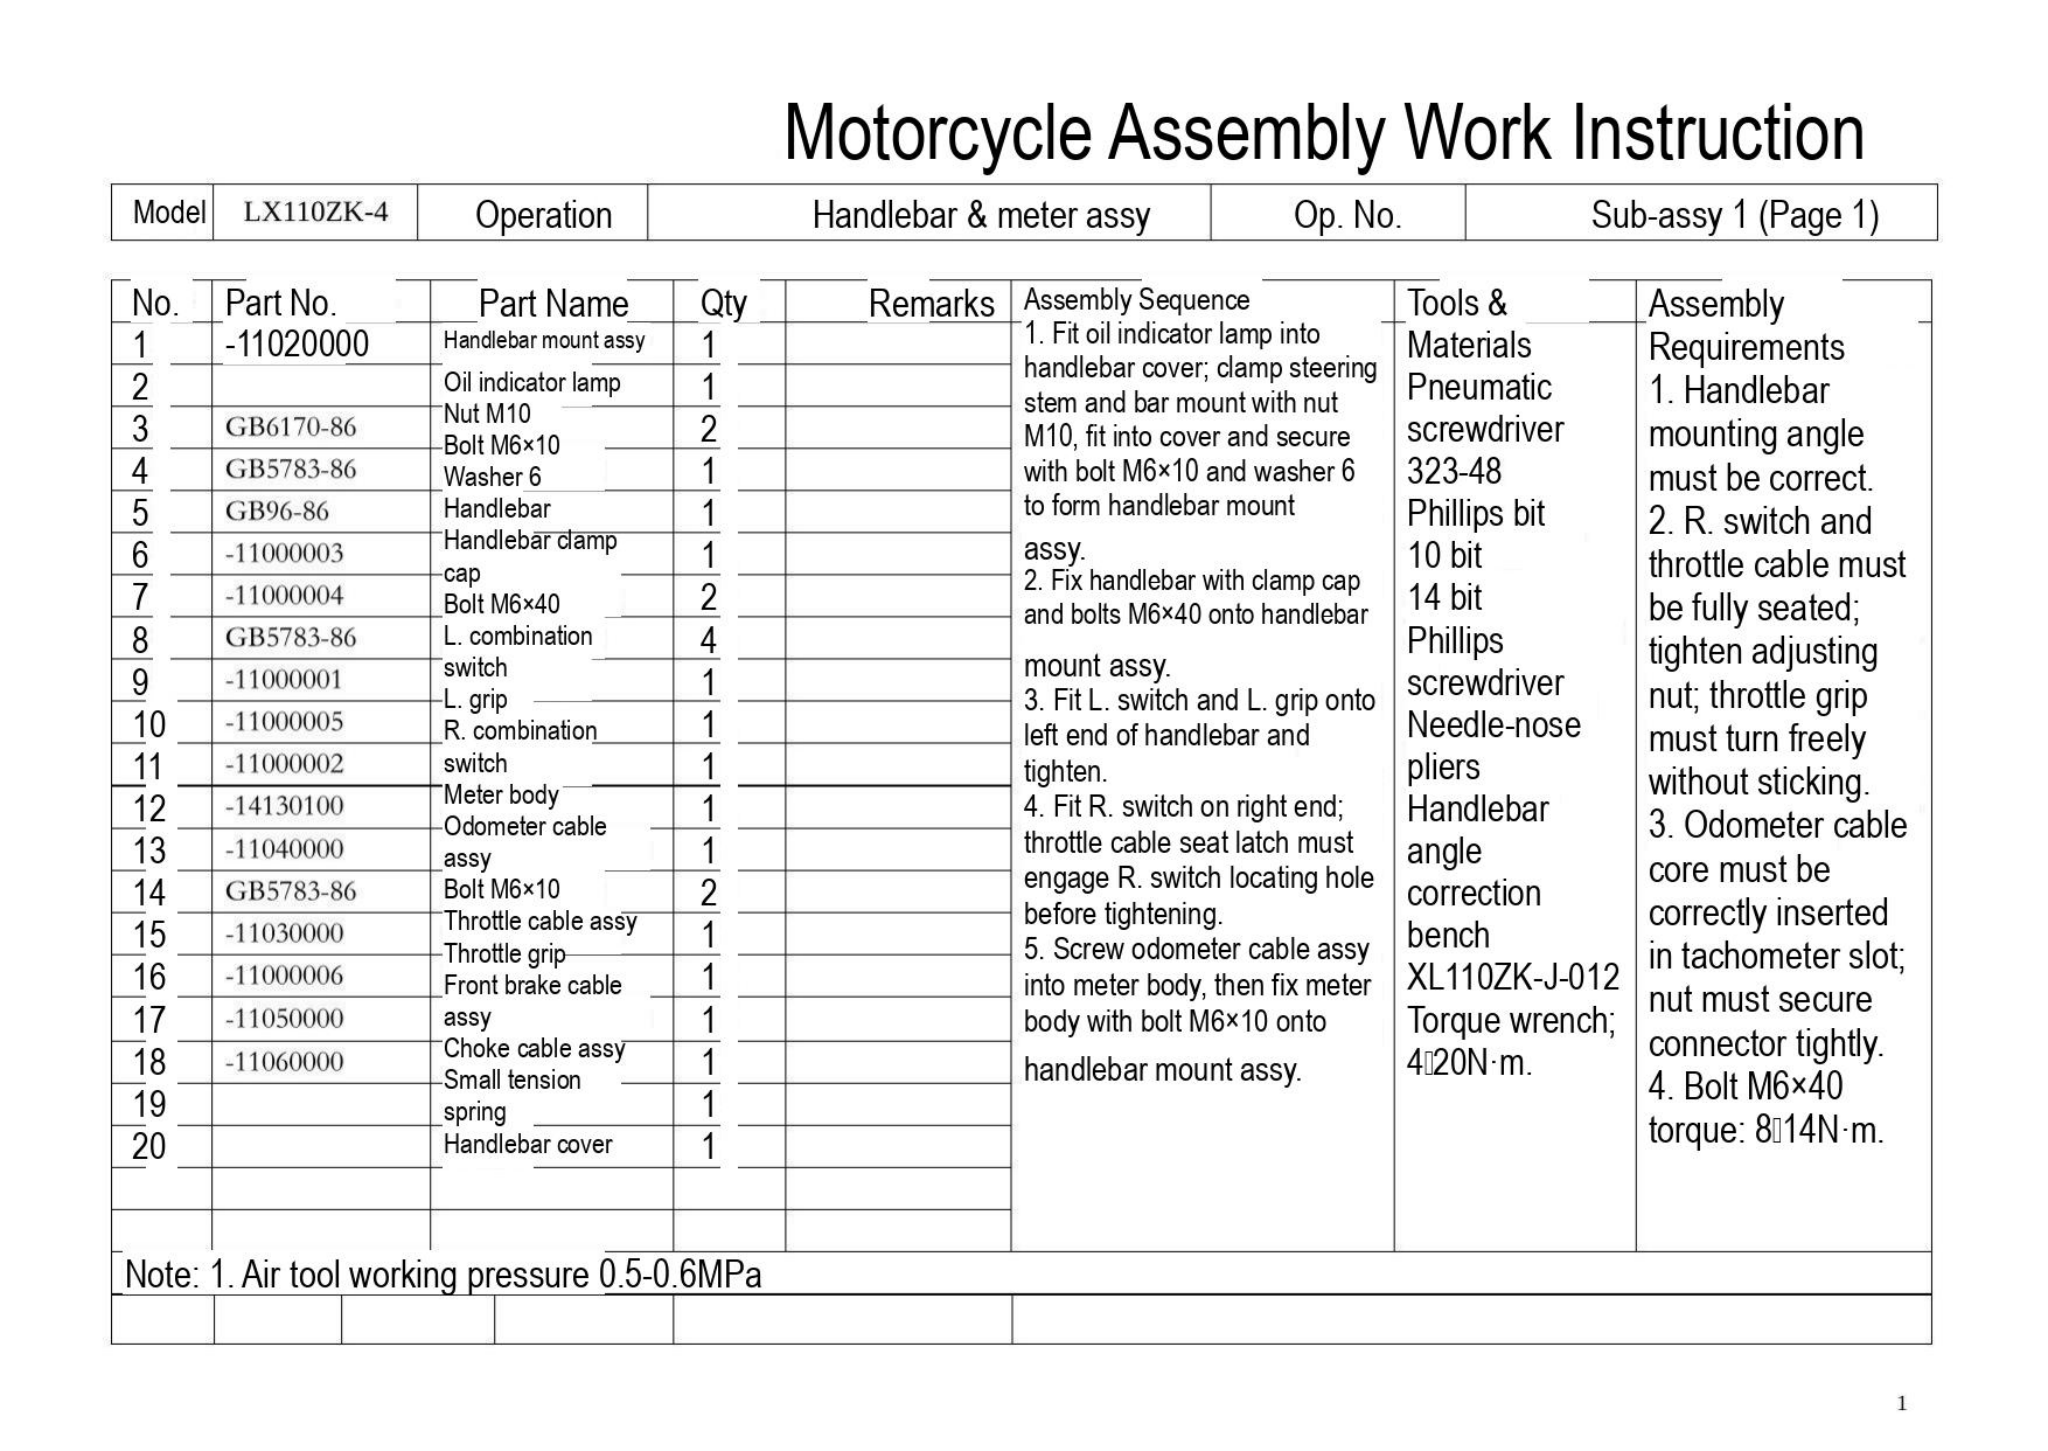# Motorcycle Assembly Work Instruction

| Model | LX110ZK-4 | Operation | Handlebar & meter assy | Op. No. | Sub-assy 1 (Page 1) |
|---|---|---|---|---|---|

| No. | Part No. | Part Name | Qty | Remarks |
|---|---|---|---|---|
| 1 | -11020000 | Handlebar mount assy | 1 | |
| 2 | | Oil indicator lamp | 1 | |
| 3 | GB6170-86 | Nut M10 | 2 | |
| 4 | GB5783-86 | Bolt M6×10 | 1 | |
| 5 | GB96-86 | Washer 6 | 1 | |
| 6 | -11000003 | Handlebar | 1 | |
| 7 | -11000004 | Handlebar clamp cap | 2 | |
| 8 | GB5783-86 | Bolt M6×40 | 4 | |
| 9 | -11000001 | L. combination switch | 1 | |
| 10 | -11000005 | L. grip | 1 | |
| 11 | -11000002 | R. combination switch | 1 | |
| 12 | -14130100 | Meter body | 1 | |
| 13 | -11040000 | Odometer cable assy | 1 | |
| 14 | GB5783-86 | Bolt M6×10 | 2 | |
| 15 | -11030000 | Throttle cable assy | 1 | |
| 16 | -11000006 | Throttle grip | 1 | |
| 17 | -11050000 | Front brake cable assy | 1 | |
| 18 | -11060000 | Choke cable assy | 1 | |
| 19 | | Small tension spring | 1 | |
| 20 | | Handlebar cover | 1 | |

**Assembly Sequence**
1. Fit oil indicator lamp into handlebar cover; clamp steering stem and bar mount with nut M10, fit into cover and secure with bolt M6×10 and washer 6 to form handlebar mount assy.
2. Fix handlebar with clamp cap and bolts M6×40 onto handlebar mount assy.
3. Fit L. switch and L. grip onto left end of handlebar and tighten.
4. Fit R. switch on right end; throttle cable seat latch must engage R. switch locating hole before tightening.
5. Screw odometer cable assy into meter body, then fix meter body with bolt M6×10 onto handlebar mount assy.

**Tools & Materials**
Pneumatic screwdriver 323-48
Phillips bit
10 bit
14 bit
Phillips screwdriver
Needle-nose pliers
Handlebar angle correction bench XL110ZK-J-012
Torque wrench; 4□20N·m.

**Assembly Requirements**
1. Handlebar mounting angle must be correct.
2. R. switch and throttle cable must be fully seated; tighten adjusting nut; throttle grip must turn freely without sticking.
3. Odometer cable core must be correctly inserted in tachometer slot; nut must secure connector tightly.
4. Bolt M6×40 torque: 8□14N·m.

Note: 1. Air tool working pressure 0.5-0.6MPa

1
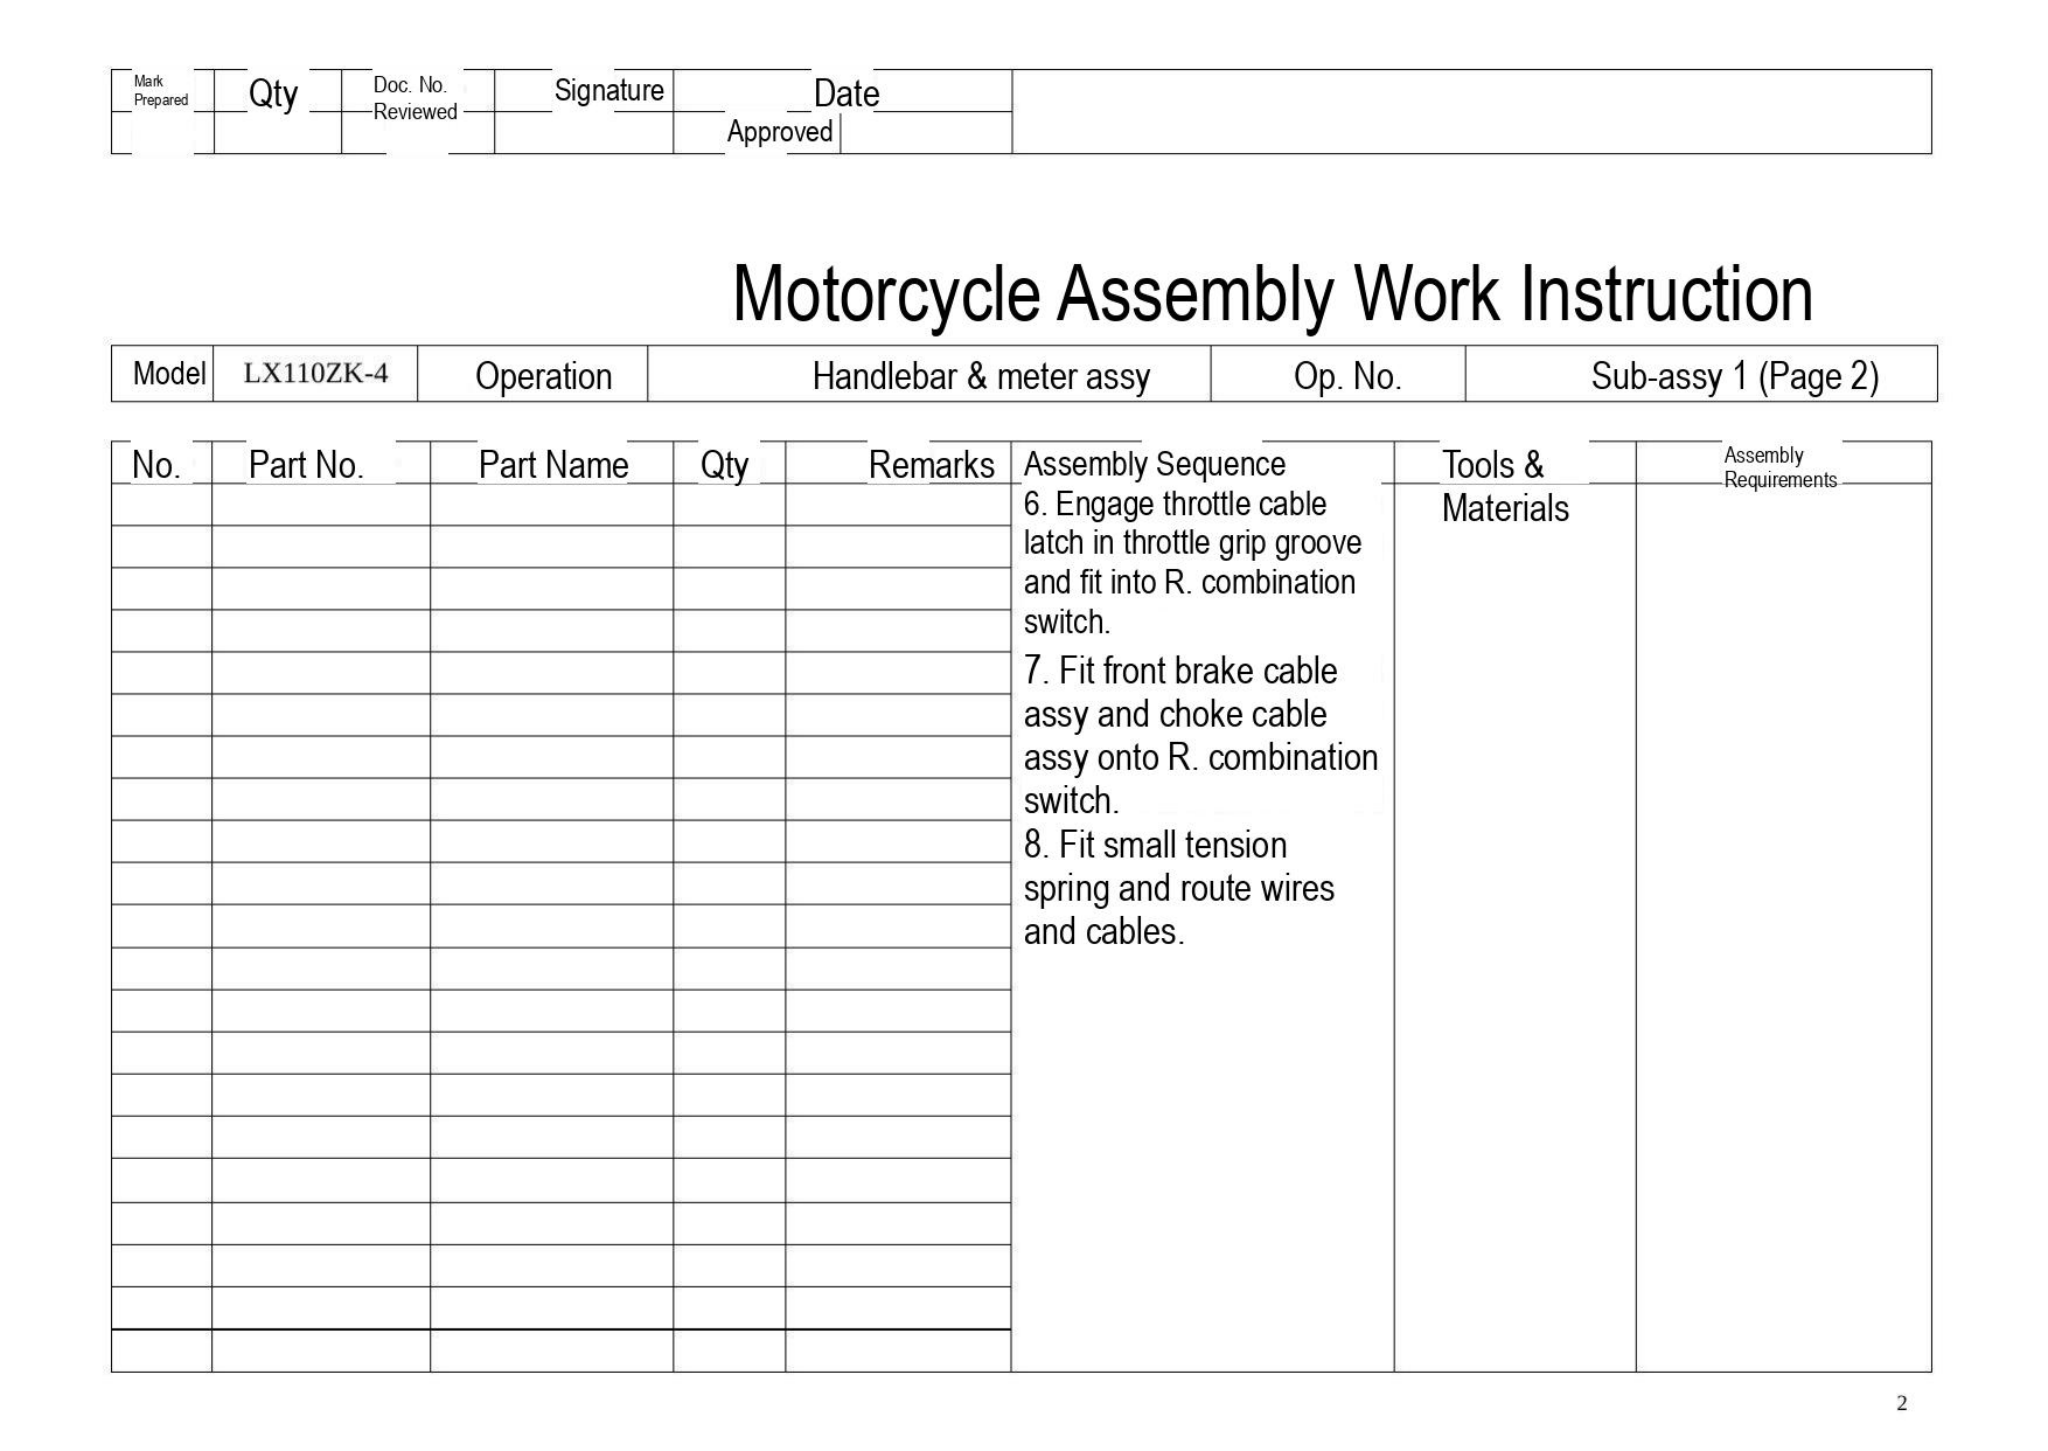| Mark Prepared | Qty | Doc. No. Reviewed | Signature | Date Approved | |
|---|---|---|---|---|---|
| | | | | | |

# Motorcycle Assembly Work Instruction

| Model | LX110ZK-4 | Operation | Handlebar & meter assy | Op. No. | Sub-assy 1 (Page 2) |
|---|---|---|---|---|---|

| No. | Part No. | Part Name | Qty | Remarks | Assembly Sequence | Tools & Materials | Assembly Requirements |
|---|---|---|---|---|---|---|---|
| | | | | | 6. Engage throttle cable latch in throttle grip groove and fit into R. combination switch.<br>7. Fit front brake cable assy and choke cable assy onto R. combination switch.<br>8. Fit small tension spring and route wires and cables. | | |

2
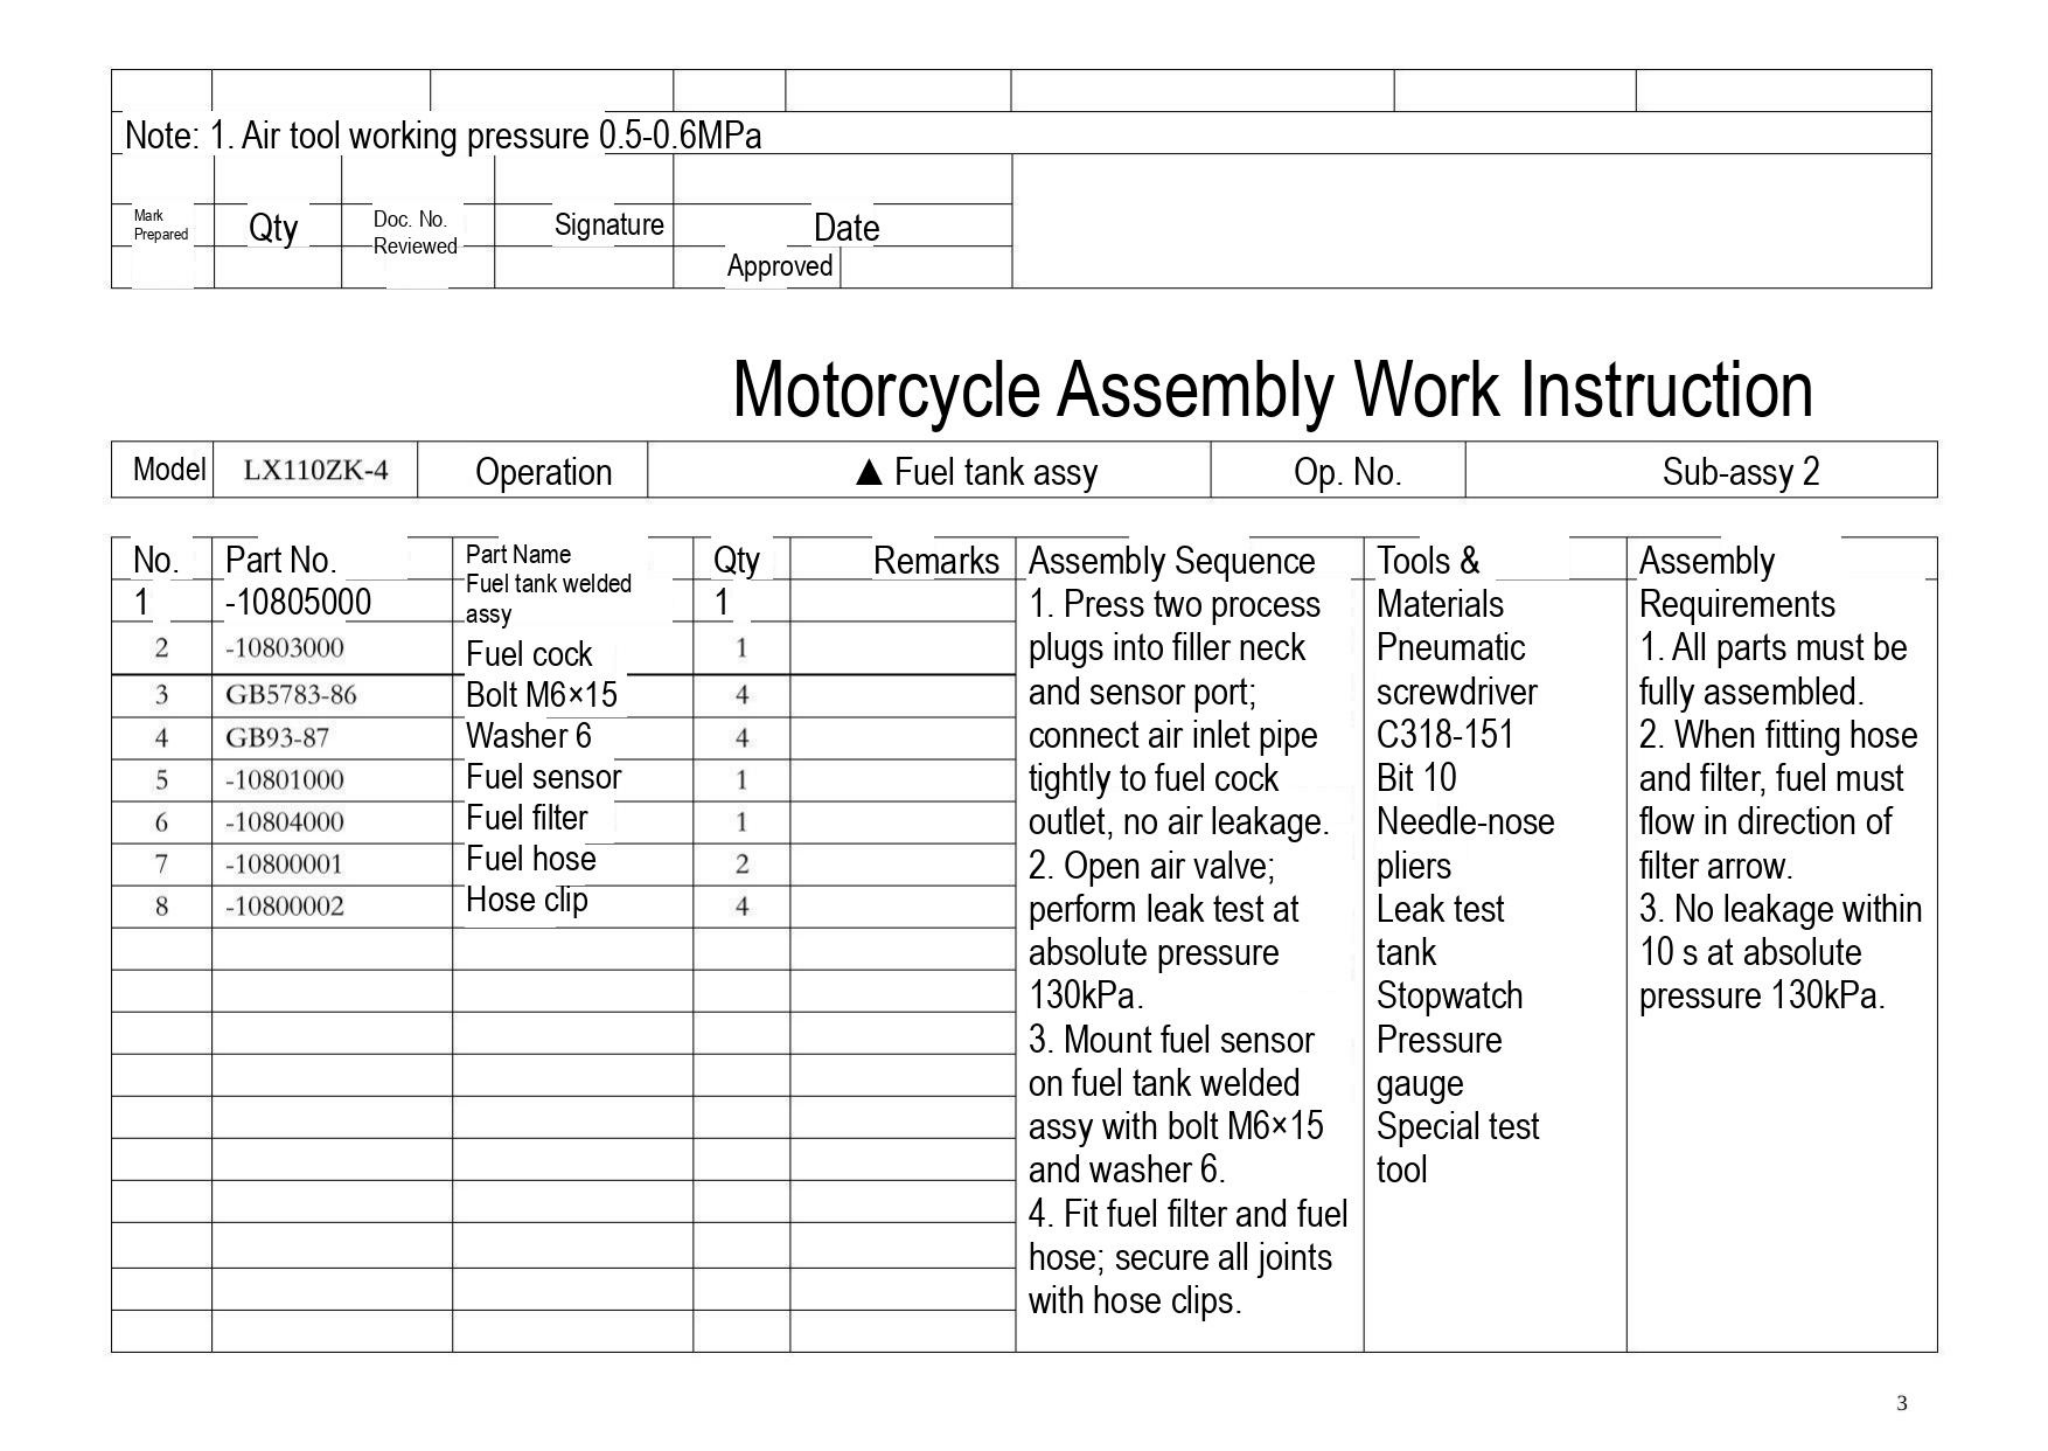| | | | | | | | |
|---|---|---|---|---|---|---|---|
| Note: 1. Air tool working pressure 0.5-0.6MPa | | | | | | | |
| Mark Prepared | Qty | Doc. No. Reviewed | Signature | Date Approved | | | |

# Motorcycle Assembly Work Instruction

| Model | LX110ZK-4 | Operation | ▲ Fuel tank assy | Op. No. | Sub-assy 2 |
|---|---|---|---|---|---|

| No. | Part No. | Part Name | Qty | Remarks | Assembly Sequence | Tools & Materials | Assembly Requirements |
|---|---|---|---|---|---|---|---|
| 1 | -10805000 | Fuel tank welded assy | 1 | | 1. Press two process plugs into filler neck and sensor port; connect air inlet pipe tightly to fuel cock outlet, no air leakage.<br>2. Open air valve; perform leak test at absolute pressure 130kPa.<br>3. Mount fuel sensor on fuel tank welded assy with bolt M6×15 and washer 6.<br>4. Fit fuel filter and fuel hose; secure all joints with hose clips. | Pneumatic screwdriver C318-151<br>Bit 10<br>Needle-nose pliers<br>Leak test tank<br>Stopwatch<br>Pressure gauge<br>Special test tool | 1. All parts must be fully assembled.<br>2. When fitting hose and filter, fuel must flow in direction of filter arrow.<br>3. No leakage within 10 s at absolute pressure 130kPa. |
| 2 | -10803000 | Fuel cock | 1 | | | | |
| 3 | GB5783-86 | Bolt M6×15 | 4 | | | | |
| 4 | GB93-87 | Washer 6 | 4 | | | | |
| 5 | -10801000 | Fuel sensor | 1 | | | | |
| 6 | -10804000 | Fuel filter | 1 | | | | |
| 7 | -10800001 | Fuel hose | 2 | | | | |
| 8 | -10800002 | Hose clip | 4 | | | | |

3
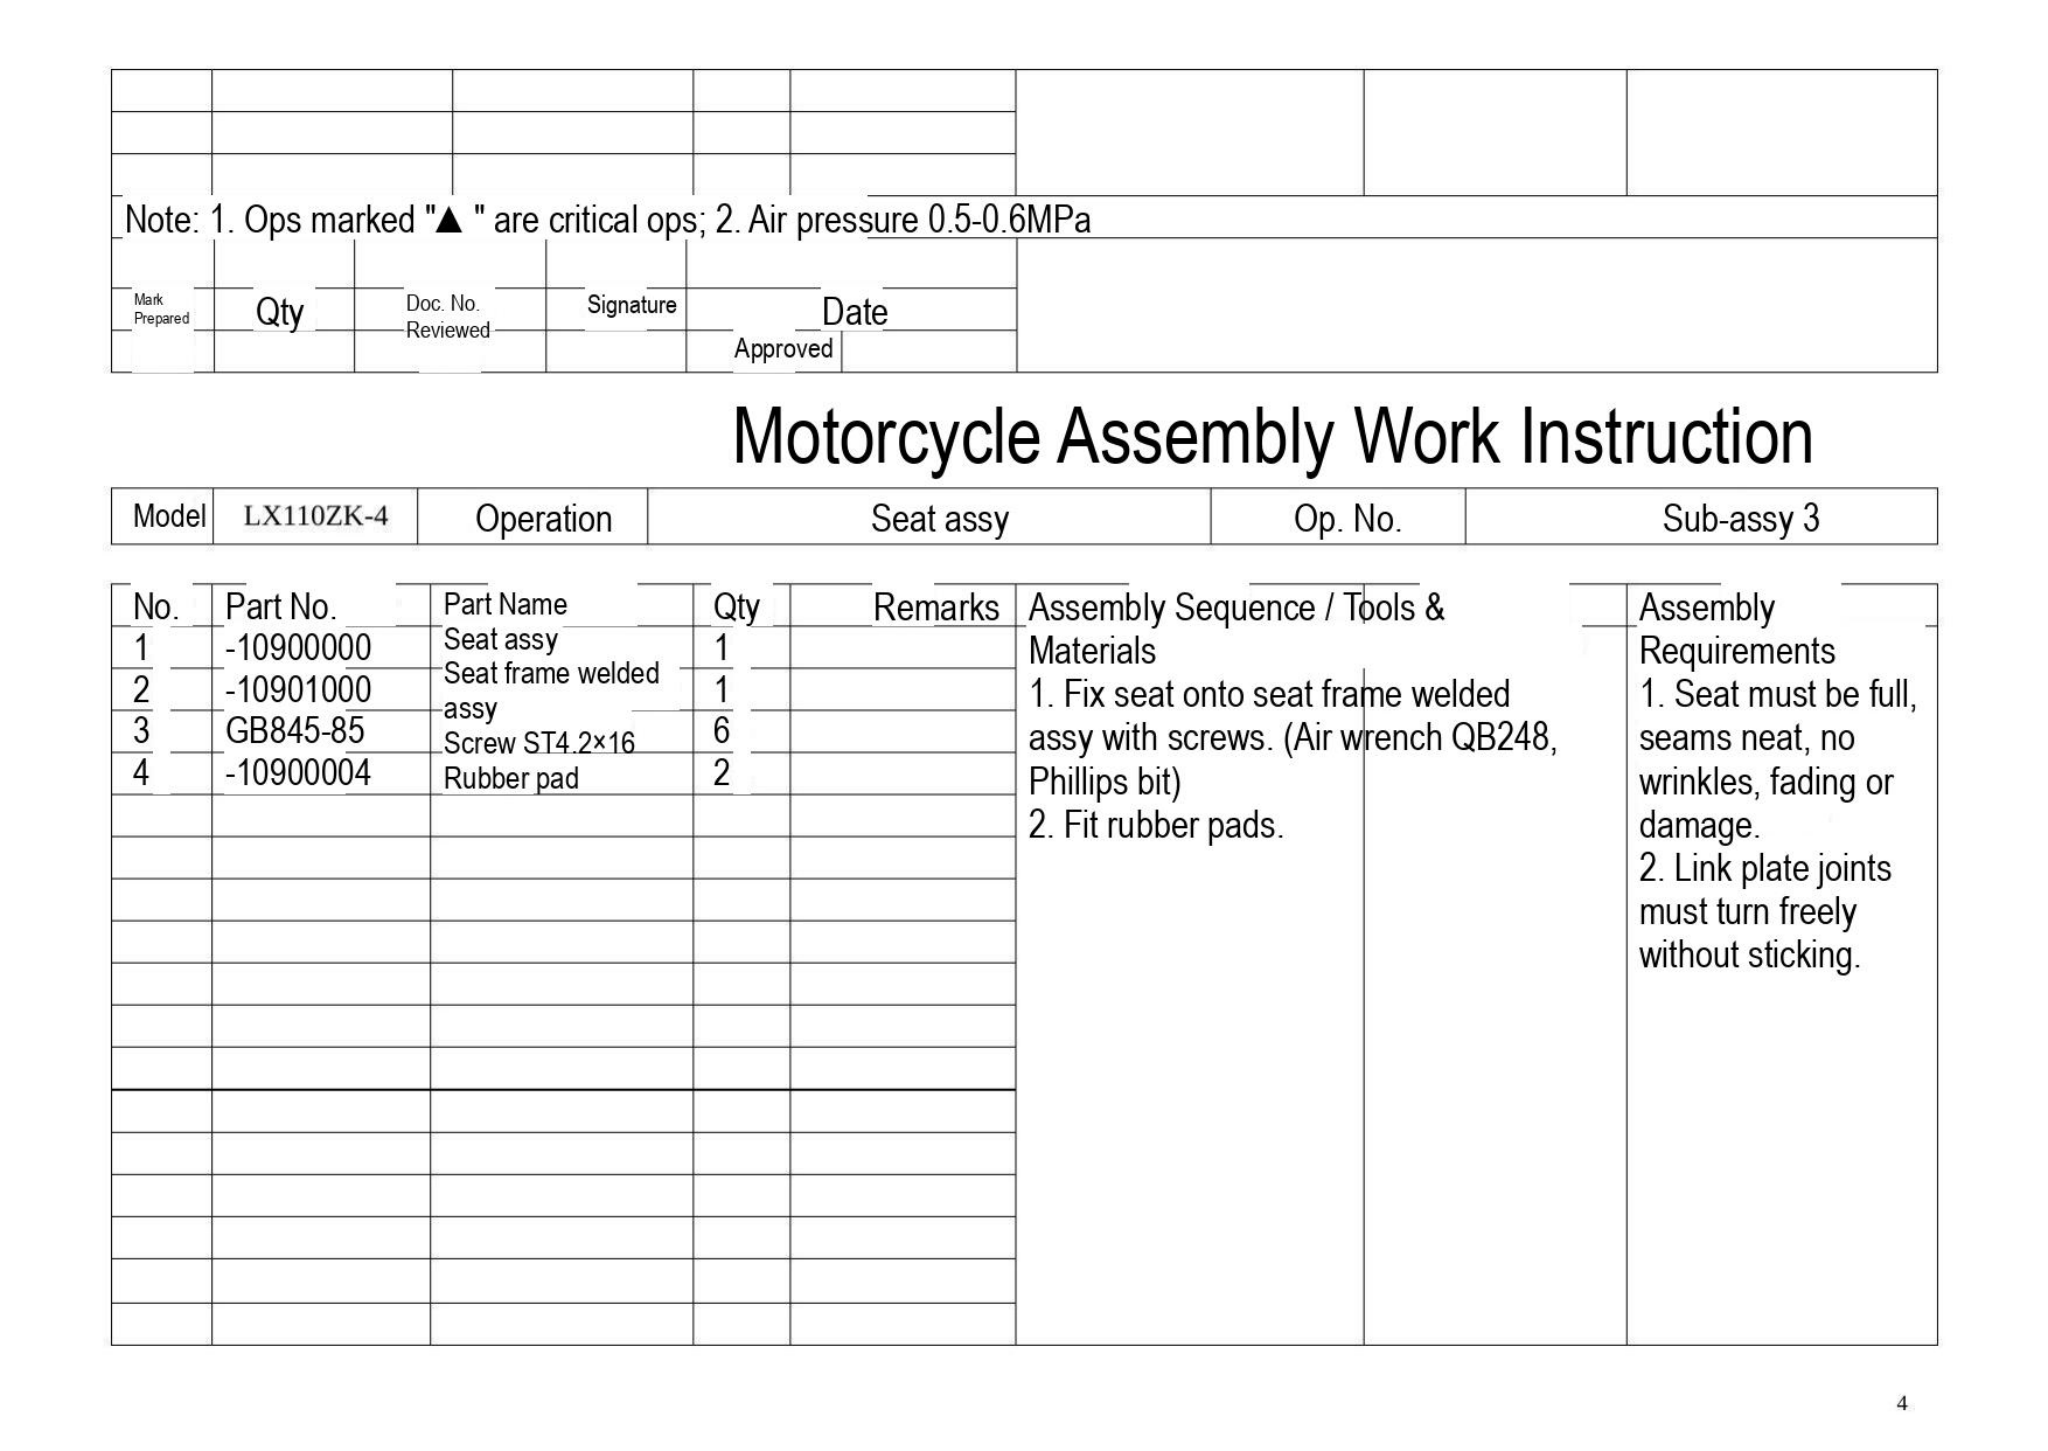Note: 1. Ops marked "▲ " are critical ops; 2. Air pressure 0.5-0.6MPa

| Mark Prepared | Qty | Doc. No. Reviewed | Signature | Date Approved |
|---|---|---|---|---|

# Motorcycle Assembly Work Instruction

| Model | LX110ZK-4 | Operation | Seat assy | Op. No. | Sub-assy 3 |
|---|---|---|---|---|---|

| No. | Part No. | Part Name | Qty | Remarks |
|---|---|---|---|---|
| 1 | -10900000 | Seat assy | 1 | |
| 2 | -10901000 | Seat frame welded assy | 1 | |
| 3 | GB845-85 | Screw ST4.2×16 | 6 | |
| 4 | -10900004 | Rubber pad | 2 | |

Assembly Sequence / Tools & Materials
1. Fix seat onto seat frame welded assy with screws. (Air wrench QB248, Phillips bit)
2. Fit rubber pads.

Assembly Requirements
1. Seat must be full, seams neat, no wrinkles, fading or damage.
2. Link plate joints must turn freely without sticking.

4
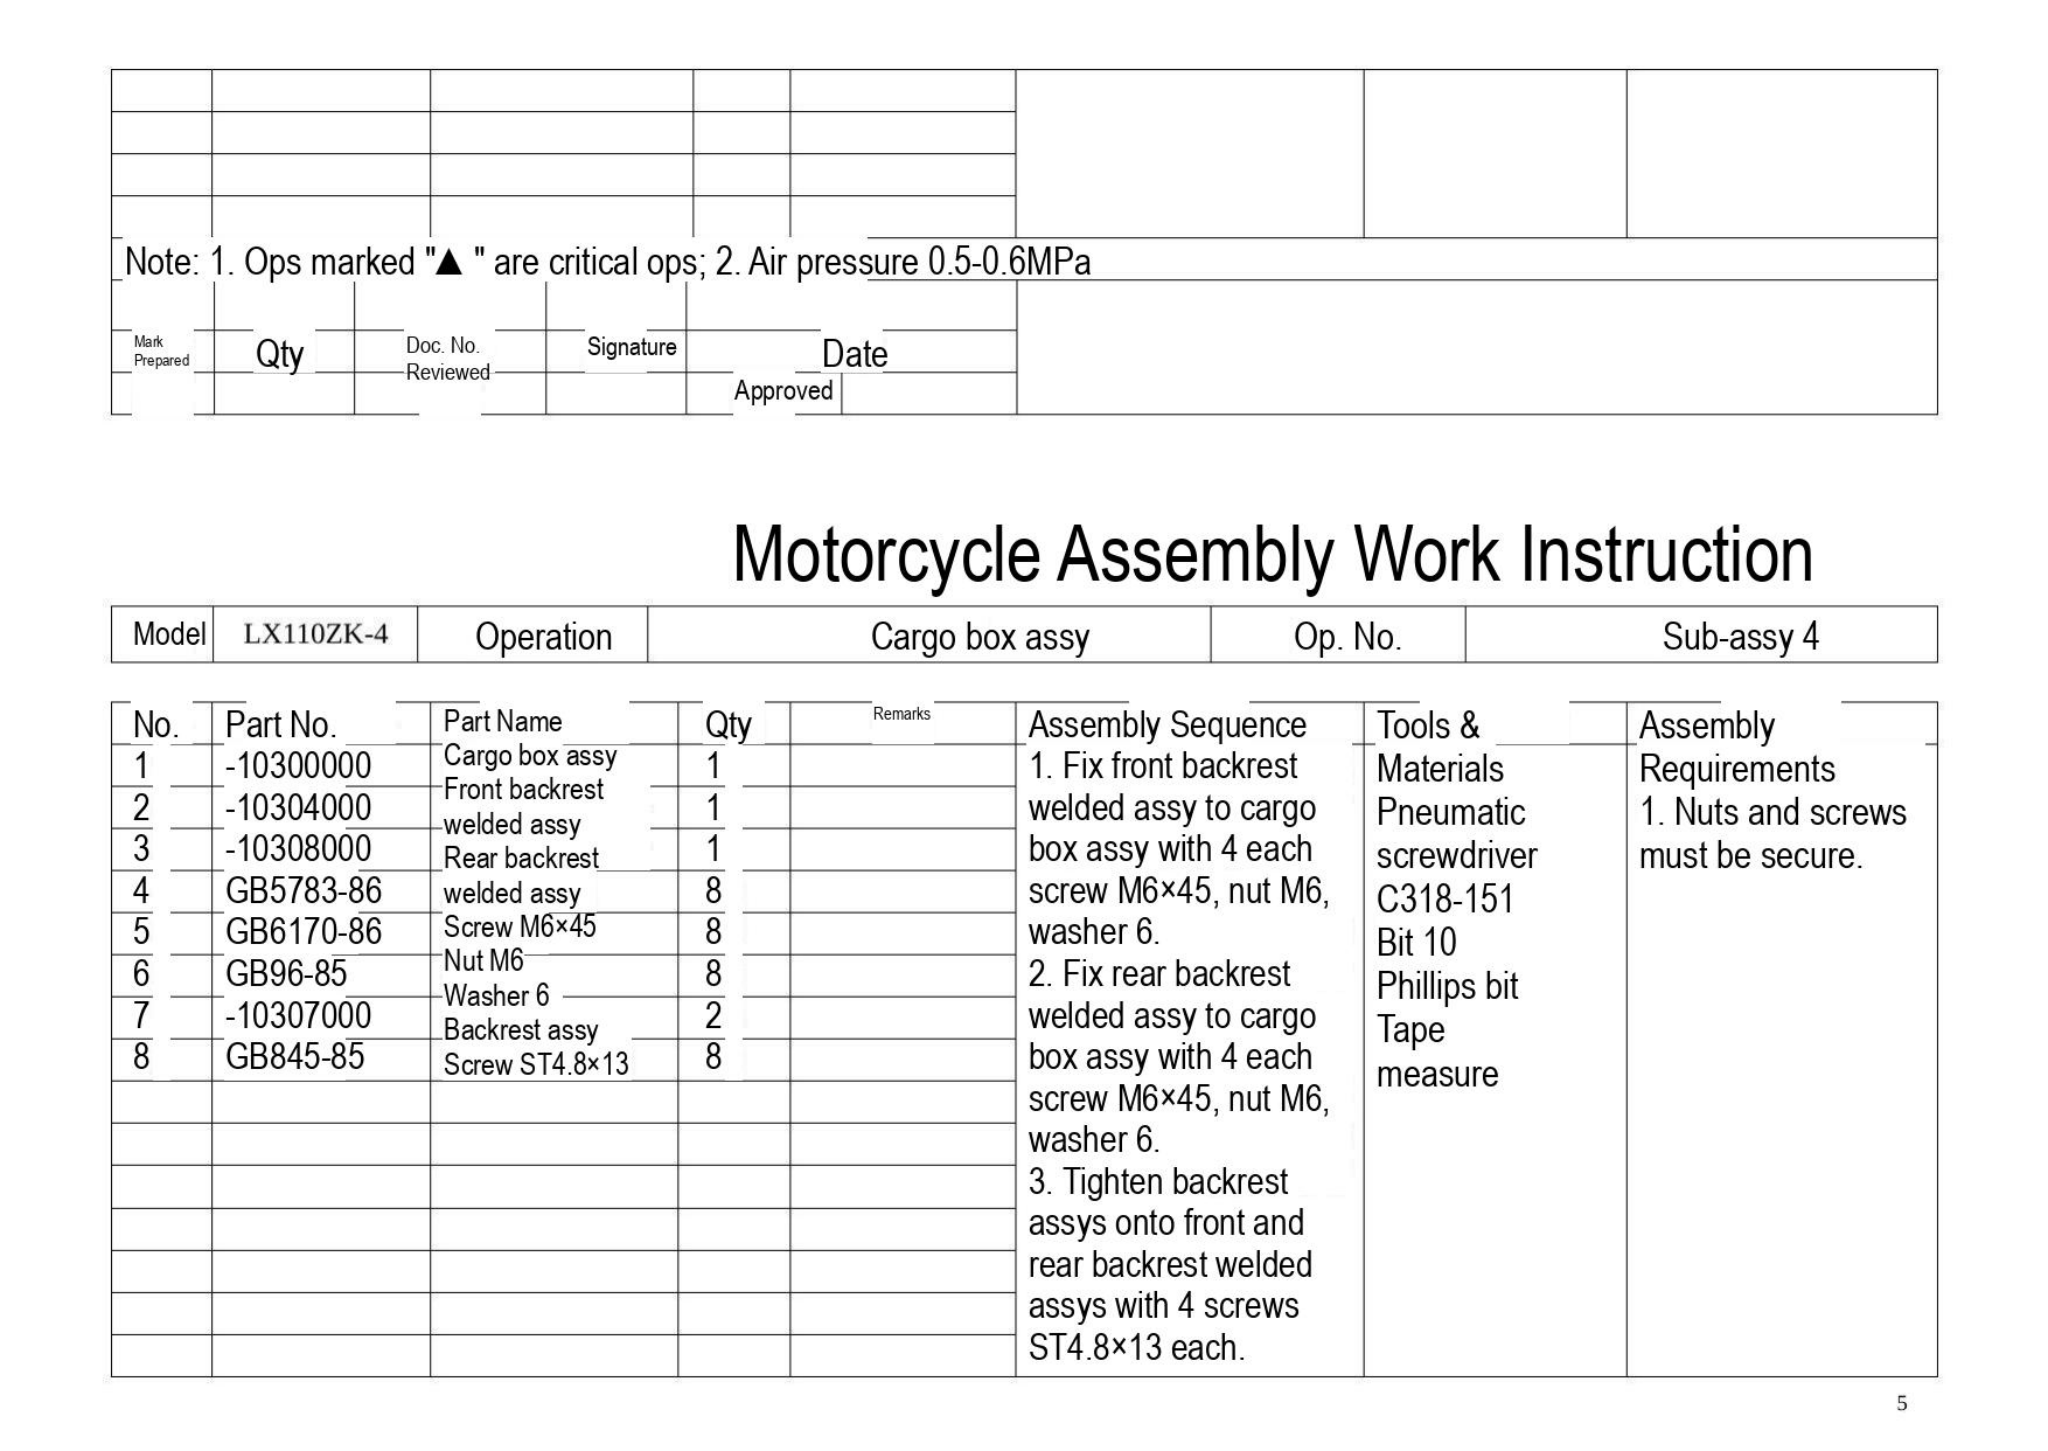Note: 1. Ops marked "▲ " are critical ops; 2. Air pressure 0.5-0.6MPa

| Mark Prepared | Qty | Doc. No. Reviewed | Signature | Date Approved |
|---|---|---|---|---|

# Motorcycle Assembly Work Instruction

| Model | LX110ZK-4 | Operation | Cargo box assy | Op. No. | Sub-assy 4 |
|---|---|---|---|---|---|

| No. | Part No. | Part Name | Qty | Remarks |
|---|---|---|---|---|
| 1 | -10300000 | Cargo box assy | 1 | |
| 2 | -10304000 | Front backrest welded assy | 1 | |
| 3 | -10308000 | Rear backrest welded assy | 1 | |
| 4 | GB5783-86 | Screw M6×45 | 8 | |
| 5 | GB6170-86 | Nut M6 | 8 | |
| 6 | GB96-85 | Washer 6 | 8 | |
| 7 | -10307000 | Backrest assy | 2 | |
| 8 | GB845-85 | Screw ST4.8×13 | 8 | |

Assembly Sequence
1. Fix front backrest welded assy to cargo box assy with 4 each screw M6×45, nut M6, washer 6.
2. Fix rear backrest welded assy to cargo box assy with 4 each screw M6×45, nut M6, washer 6.
3. Tighten backrest assys onto front and rear backrest welded assys with 4 screws ST4.8×13 each.

Tools & Materials
Pneumatic screwdriver C318-151
Bit 10
Phillips bit
Tape measure

Assembly Requirements
1. Nuts and screws must be secure.

5
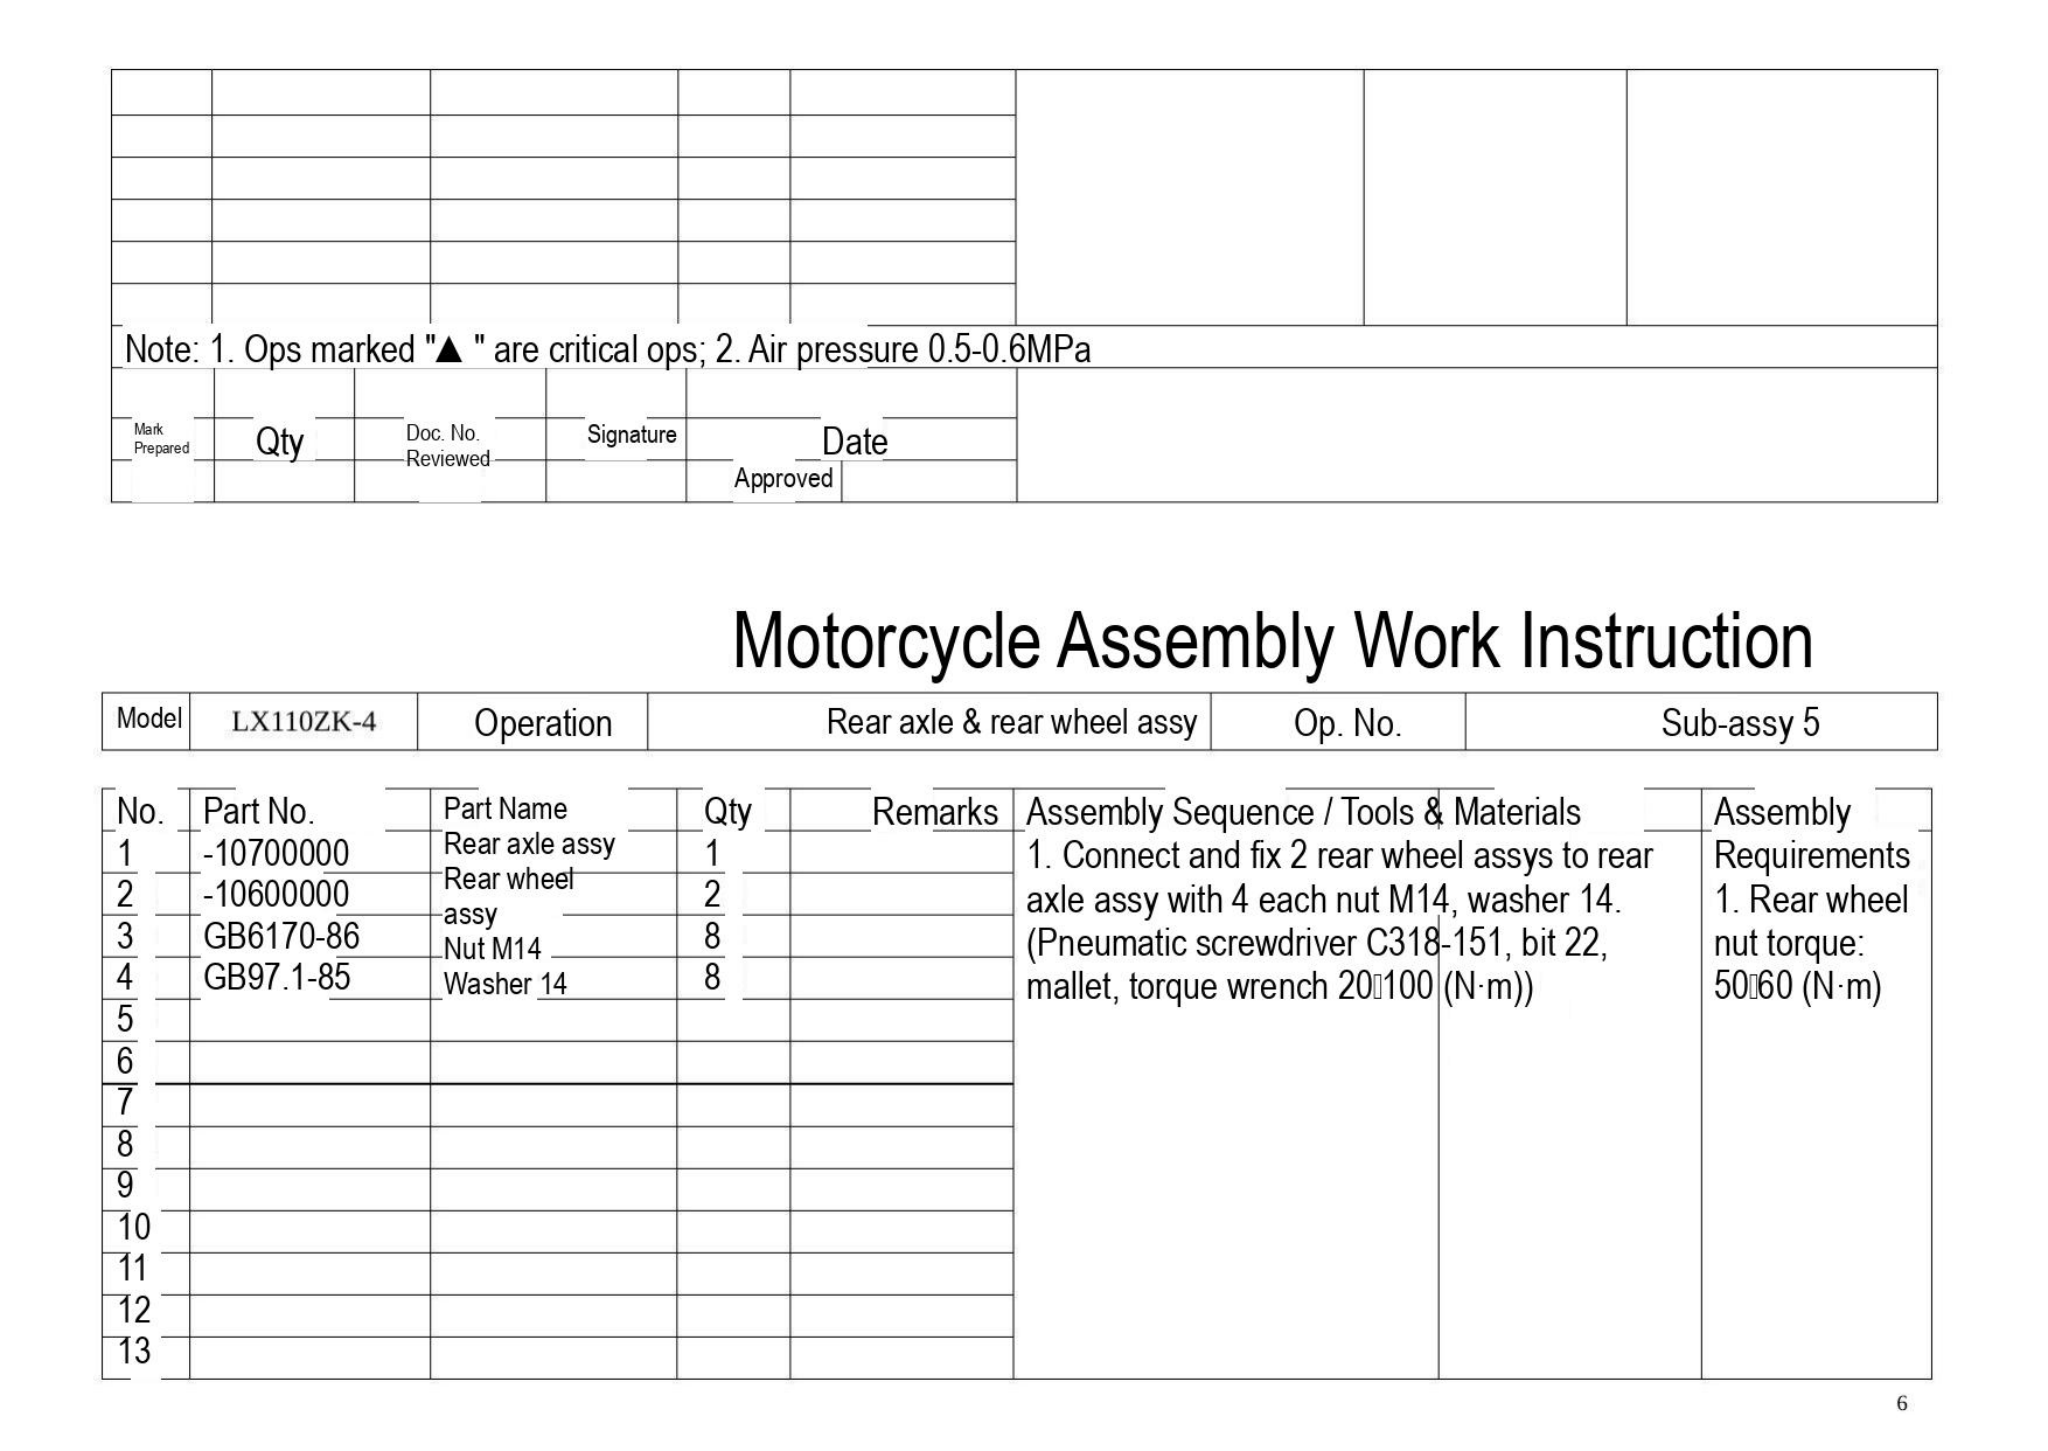Note: 1. Ops marked "▲ " are critical ops; 2. Air pressure 0.5-0.6MPa

| Mark Prepared | Qty | Doc. No. Reviewed | Signature | Date Approved |
|---|---|---|---|---|

# Motorcycle Assembly Work Instruction

| Model | LX110ZK-4 | Operation | Rear axle & rear wheel assy | Op. No. | Sub-assy 5 |
|---|---|---|---|---|---|

| No. | Part No. | Part Name | Qty | Remarks |
|---|---|---|---|---|
| 1 | -10700000 | Rear axle assy | 1 | |
| 2 | -10600000 | Rear wheel assy | 2 | |
| 3 | GB6170-86 | Nut M14 | 8 | |
| 4 | GB97.1-85 | Washer 14 | 8 | |
| 5 | | | | |
| 6 | | | | |
| 7 | | | | |
| 8 | | | | |
| 9 | | | | |
| 10 | | | | |
| 11 | | | | |
| 12 | | | | |
| 13 | | | | |

Assembly Sequence / Tools & Materials

1. Connect and fix 2 rear wheel assys to rear axle assy with 4 each nut M14, washer 14. (Pneumatic screwdriver C318-151, bit 22, mallet, torque wrench 20100 (N·m))

Assembly Requirements

1. Rear wheel nut torque: 5060 (N·m)

6
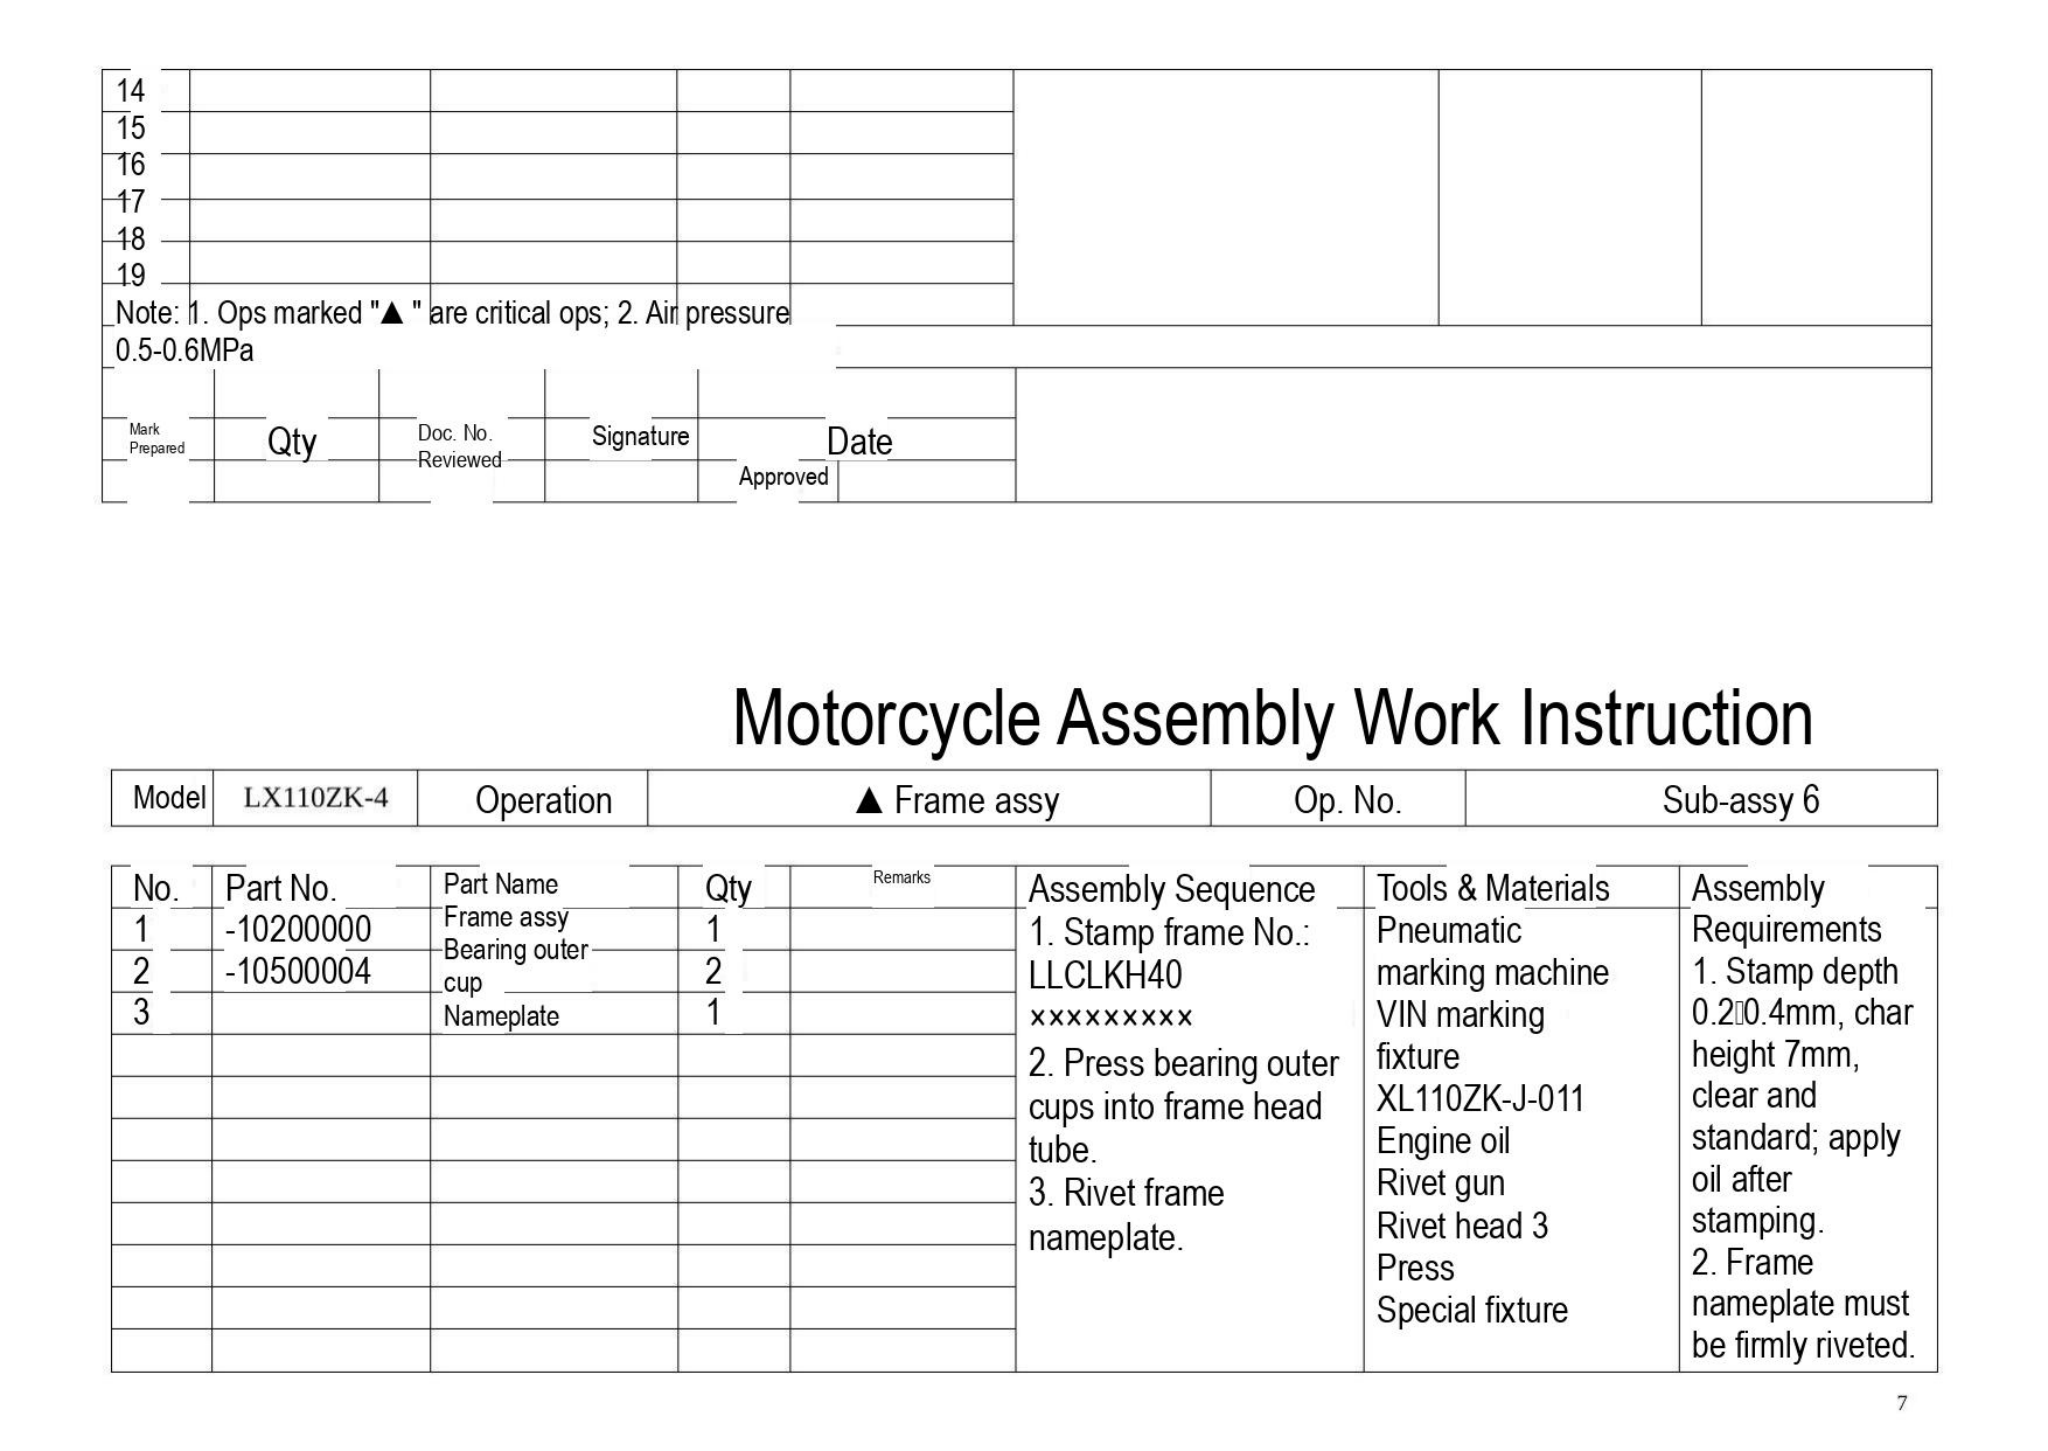| 14 | | | | | | | |
|---|---|---|---|---|---|---|---|
| 15 | | | | | | | |
| 16 | | | | | | | |
| 17 | | | | | | | |
| 18 | | | | | | | |
| 19 | | | | | | | |

Note: 1. Ops marked "▲ " are critical ops; 2. Air pressure 0.5-0.6MPa

| Mark<br>Prepared | Qty | Doc. No.<br>Reviewed | Signature | Date<br>Approved | |
|---|---|---|---|---|---|
| | | | | | |

# Motorcycle Assembly Work Instruction

| Model | LX110ZK-4 | Operation | ▲ Frame assy | Op. No. | Sub-assy 6 |
|---|---|---|---|---|---|

| No. | Part No. | Part Name | Qty | Remarks | Assembly Sequence | Tools & Materials | Assembly Requirements |
|---|---|---|---|---|---|---|---|
| 1 | -10200000 | Frame assy | 1 | | 1. Stamp frame No.: LLCLKH40 ××××××××× <br>2. Press bearing outer cups into frame head tube.<br>3. Rivet frame nameplate. | Pneumatic marking machine<br>VIN marking fixture XL110ZK-J-011<br>Engine oil<br>Rivet gun<br>Rivet head 3<br>Press<br>Special fixture | 1. Stamp depth 0.2 0.4mm, char height 7mm, clear and standard; apply oil after stamping.<br>2. Frame nameplate must be firmly riveted. |
| 2 | -10500004 | Bearing outer cup | 2 | | | | |
| 3 | | Nameplate | 1 | | | | |
| | | | | | | | |
| | | | | | | | |
| | | | | | | | |
| | | | | | | | |
| | | | | | | | |
| | | | | | | | |
| | | | | | | | |

7